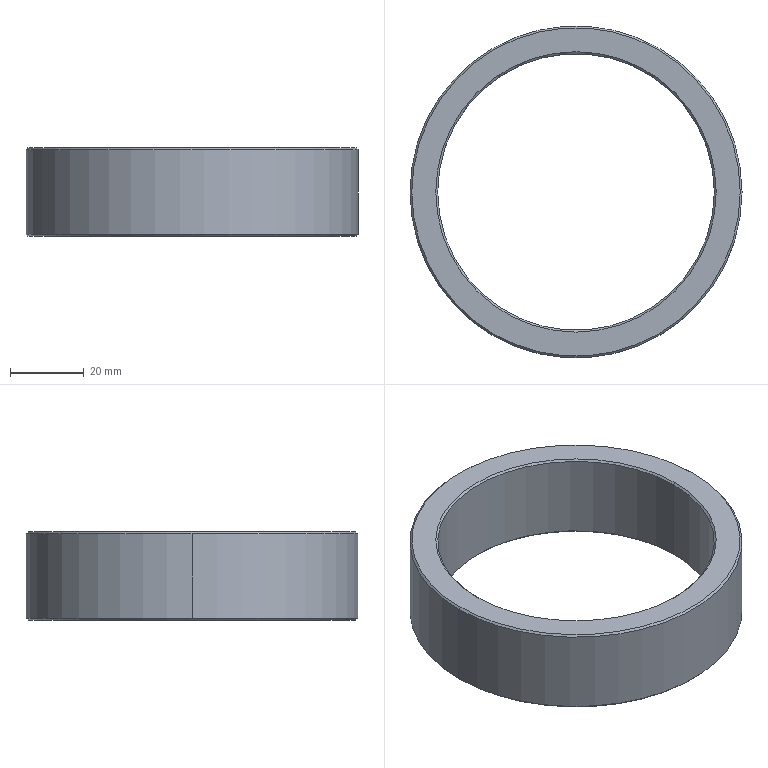Part | SolidWorks | features Chamfer 1, Extrusion 1 | 1 solid | 14 faces | box 90 x 90 x 24 mm | volume 46523 mm3 | cone 8 | cylinder 4 | plane 2 | commonest cylinder face diameters 75 x2 90 x2
STEP:
#1=CARTESIAN_POINT('',(44.5,0.,24.));
#2=VERTEX_POINT('',#1);
#3=CARTESIAN_POINT('',(-44.5,0.,24.));
#4=VERTEX_POINT('',#3);
#5=CARTESIAN_POINT('',(0.,0.,24.));
#6=DIRECTION('',(0.,0.,1.));
#7=DIRECTION('',(1.,0.,0.));
#8=AXIS2_PLACEMENT_3D('',#5,#6,#7);
#9=CIRCLE('',#8,44.5);
#10=EDGE_CURVE('',#2,#4,#9,.T.);
#11=ORIENTED_EDGE('',*,*,#10,.F.);
#12=CARTESIAN_POINT('',(45.,0.,23.5));
#13=VERTEX_POINT('',#12);
#14=CARTESIAN_POINT('',(44.5,0.,24.));
#15=DIRECTION('',(0.7071,0.,-0.7071));
#16=VECTOR('',#15,1000.);
#17=LINE('',#14,#16);
#18=EDGE_CURVE('',#2,#13,#17,.T.);
#19=ORIENTED_EDGE('',*,*,#18,.T.);
#20=CARTESIAN_POINT('',(-45.,0.,23.5));
#21=VERTEX_POINT('',#20);
#22=CARTESIAN_POINT('',(0.,0.,23.5));
#23=DIRECTION('',(0.,0.,-1.));
#24=DIRECTION('',(1.,0.,0.));
#25=AXIS2_PLACEMENT_3D('',#22,#23,#24);
#26=CIRCLE('',#25,45.);
#27=EDGE_CURVE('',#21,#13,#26,.T.);
#28=ORIENTED_EDGE('',*,*,#27,.F.);
#29=CARTESIAN_POINT('',(-44.5,0.,24.));
#30=DIRECTION('',(-0.7071,0.,-0.7071));
#31=VECTOR('',#30,1000.);
#32=LINE('',#29,#31);
#33=EDGE_CURVE('',#4,#21,#32,.T.);
#34=ORIENTED_EDGE('',*,*,#33,.F.);
#35=EDGE_LOOP('',(#11,#19,#28,#34));
#36=FACE_OUTER_BOUND('',#35,.T.);
#37=CARTESIAN_POINT('',(0.,0.,24.));
#38=DIRECTION('',(0.,0.,-1.));
#39=DIRECTION('',(-1.,0.,0.));
#40=AXIS2_PLACEMENT_3D('',#37,#38,#39);
#41=CONICAL_SURFACE('',#40,44.5,0.7854);
#42=ADVANCED_FACE('',(#36),#41,.T.);
#43=CARTESIAN_POINT('',(-37.5,0.,23.5));
#44=VERTEX_POINT('',#43);
#45=CARTESIAN_POINT('',(37.5,0.,23.5));
#46=VERTEX_POINT('',#45);
#47=CARTESIAN_POINT('',(0.,0.,23.5));
#48=DIRECTION('',(0.,0.,1.));
#49=DIRECTION('',(1.,0.,0.));
#50=AXIS2_PLACEMENT_3D('',#47,#48,#49);
#51=CIRCLE('',#50,37.5);
#52=EDGE_CURVE('',#44,#46,#51,.T.);
#53=ORIENTED_EDGE('',*,*,#52,.F.);
#54=CARTESIAN_POINT('',(-38.,0.,24.));
#55=VERTEX_POINT('',#54);
#56=CARTESIAN_POINT('',(-37.5,0.,23.5));
#57=DIRECTION('',(-0.7071,0.,0.7071));
#58=VECTOR('',#57,1000.);
#59=LINE('',#56,#58);
#60=EDGE_CURVE('',#44,#55,#59,.T.);
#61=ORIENTED_EDGE('',*,*,#60,.T.);
#62=CARTESIAN_POINT('',(38.,0.,24.));
#63=VERTEX_POINT('',#62);
#64=CARTESIAN_POINT('',(0.,0.,24.));
#65=DIRECTION('',(0.,0.,-1.));
#66=DIRECTION('',(1.,0.,0.));
#67=AXIS2_PLACEMENT_3D('',#64,#65,#66);
#68=CIRCLE('',#67,38.);
#69=EDGE_CURVE('',#63,#55,#68,.T.);
#70=ORIENTED_EDGE('',*,*,#69,.F.);
#71=CARTESIAN_POINT('',(37.5,0.,23.5));
#72=DIRECTION('',(0.7071,0.,0.7071));
#73=VECTOR('',#72,1000.);
#74=LINE('',#71,#73);
#75=EDGE_CURVE('',#46,#63,#74,.T.);
#76=ORIENTED_EDGE('',*,*,#75,.F.);
#77=EDGE_LOOP('',(#53,#61,#70,#76));
#78=FACE_OUTER_BOUND('',#77,.T.);
#79=CARTESIAN_POINT('',(0.,0.,23.5));
#80=DIRECTION('',(0.,0.,1.));
#81=DIRECTION('',(1.,0.,0.));
#82=AXIS2_PLACEMENT_3D('',#79,#80,#81);
#83=CONICAL_SURFACE('',#82,37.5,0.7854);
#84=ADVANCED_FACE('',(#78),#83,.F.);
#85=CARTESIAN_POINT('',(-44.5,0.,0.));
#86=VERTEX_POINT('',#85);
#87=CARTESIAN_POINT('',(44.5,0.,0.));
#88=VERTEX_POINT('',#87);
#89=CARTESIAN_POINT('',(0.,0.,0.));
#90=DIRECTION('',(0.,0.,-1.));
#91=DIRECTION('',(1.,0.,0.));
#92=AXIS2_PLACEMENT_3D('',#89,#90,#91);
#93=CIRCLE('',#92,44.5);
#94=EDGE_CURVE('',#86,#88,#93,.T.);
#95=ORIENTED_EDGE('',*,*,#94,.F.);
#96=CARTESIAN_POINT('',(-45.,0.,0.5));
#97=VERTEX_POINT('',#96);
#98=CARTESIAN_POINT('',(-45.,0.,0.5));
#99=DIRECTION('',(-0.7071,0.,0.7071));
#100=VECTOR('',#99,1000.);
#101=LINE('',#98,#100);
#102=EDGE_CURVE('',#86,#97,#101,.T.);
#103=ORIENTED_EDGE('',*,*,#102,.T.);
#104=CARTESIAN_POINT('',(45.,0.,0.5));
#105=VERTEX_POINT('',#104);
#106=CARTESIAN_POINT('',(0.,0.,0.5));
#107=DIRECTION('',(0.,0.,1.));
#108=DIRECTION('',(1.,0.,0.));
#109=AXIS2_PLACEMENT_3D('',#106,#107,#108);
#110=CIRCLE('',#109,45.);
#111=EDGE_CURVE('',#105,#97,#110,.T.);
#112=ORIENTED_EDGE('',*,*,#111,.F.);
#113=CARTESIAN_POINT('',(45.,0.,0.5));
#114=DIRECTION('',(0.7071,0.,0.7071));
#115=VECTOR('',#114,1000.);
#116=LINE('',#113,#115);
#117=EDGE_CURVE('',#88,#105,#116,.T.);
#118=ORIENTED_EDGE('',*,*,#117,.F.);
#119=EDGE_LOOP('',(#95,#103,#112,#118));
#120=FACE_OUTER_BOUND('',#119,.T.);
#121=CARTESIAN_POINT('',(0.,0.,0.5));
#122=DIRECTION('',(0.,0.,1.));
#123=DIRECTION('',(1.,0.,0.));
#124=AXIS2_PLACEMENT_3D('',#121,#122,#123);
#125=CONICAL_SURFACE('',#124,45.,0.7854);
#126=ADVANCED_FACE('',(#120),#125,.T.);
#127=CARTESIAN_POINT('',(37.5,0.,0.5));
#128=VERTEX_POINT('',#127);
#129=CARTESIAN_POINT('',(-37.5,0.,0.5));
#130=VERTEX_POINT('',#129);
#131=CARTESIAN_POINT('',(0.,0.,0.5));
#132=DIRECTION('',(0.,0.,-1.));
#133=DIRECTION('',(1.,0.,0.));
#134=AXIS2_PLACEMENT_3D('',#131,#132,#133);
#135=CIRCLE('',#134,37.5);
#136=EDGE_CURVE('',#128,#130,#135,.T.);
#137=ORIENTED_EDGE('',*,*,#136,.F.);
#138=CARTESIAN_POINT('',(38.,0.,0.));
#139=VERTEX_POINT('',#138);
#140=CARTESIAN_POINT('',(38.,0.,0.));
#141=DIRECTION('',(0.7071,0.,-0.7071));
#142=VECTOR('',#141,1000.);
#143=LINE('',#140,#142);
#144=EDGE_CURVE('',#128,#139,#143,.T.);
#145=ORIENTED_EDGE('',*,*,#144,.T.);
#146=CARTESIAN_POINT('',(-38.,0.,0.));
#147=VERTEX_POINT('',#146);
#148=CARTESIAN_POINT('',(0.,0.,0.));
#149=DIRECTION('',(0.,0.,1.));
#150=DIRECTION('',(1.,0.,0.));
#151=AXIS2_PLACEMENT_3D('',#148,#149,#150);
#152=CIRCLE('',#151,38.);
#153=EDGE_CURVE('',#147,#139,#152,.T.);
#154=ORIENTED_EDGE('',*,*,#153,.F.);
#155=CARTESIAN_POINT('',(-38.,0.,0.));
#156=DIRECTION('',(-0.7071,0.,-0.7071));
#157=VECTOR('',#156,1000.);
#158=LINE('',#155,#157);
#159=EDGE_CURVE('',#130,#147,#158,.T.);
#160=ORIENTED_EDGE('',*,*,#159,.F.);
#161=EDGE_LOOP('',(#137,#145,#154,#160));
#162=FACE_OUTER_BOUND('',#161,.T.);
#163=CARTESIAN_POINT('',(0.,0.,0.));
#164=DIRECTION('',(0.,0.,-1.));
#165=DIRECTION('',(-1.,0.,0.));
#166=AXIS2_PLACEMENT_3D('',#163,#164,#165);
#167=CONICAL_SURFACE('',#166,38.,0.7854);
#168=ADVANCED_FACE('',(#162),#167,.F.);
#169=ORIENTED_EDGE('',*,*,#52,.T.);
#170=CARTESIAN_POINT('',(37.5,0.,24.));
#171=DIRECTION('',(0.,0.,-1.));
#172=VECTOR('',#171,1000.);
#173=LINE('',#170,#172);
#174=EDGE_CURVE('',#46,#128,#173,.T.);
#175=ORIENTED_EDGE('',*,*,#174,.T.);
#176=ORIENTED_EDGE('',*,*,#136,.T.);
#177=CARTESIAN_POINT('',(-37.5,0.,24.));
#178=DIRECTION('',(0.,0.,-1.));
#179=VECTOR('',#178,1000.);
#180=LINE('',#177,#179);
#181=EDGE_CURVE('',#44,#130,#180,.T.);
#182=ORIENTED_EDGE('',*,*,#181,.F.);
#183=EDGE_LOOP('',(#169,#175,#176,#182));
#184=FACE_OUTER_BOUND('',#183,.T.);
#185=CARTESIAN_POINT('',(0.,0.,24.));
#186=DIRECTION('',(0.,0.,-1.));
#187=DIRECTION('',(-1.,0.,0.));
#188=AXIS2_PLACEMENT_3D('',#185,#186,#187);
#189=CYLINDRICAL_SURFACE('',#188,37.5);
#190=ADVANCED_FACE('',(#184),#189,.F.);
#191=ORIENTED_EDGE('',*,*,#27,.T.);
#192=CARTESIAN_POINT('',(45.,0.,24.));
#193=DIRECTION('',(0.,0.,-1.));
#194=VECTOR('',#193,1000.);
#195=LINE('',#192,#194);
#196=EDGE_CURVE('',#13,#105,#195,.T.);
#197=ORIENTED_EDGE('',*,*,#196,.T.);
#198=ORIENTED_EDGE('',*,*,#111,.T.);
#199=CARTESIAN_POINT('',(-45.,0.,24.));
#200=DIRECTION('',(0.,0.,-1.));
#201=VECTOR('',#200,1000.);
#202=LINE('',#199,#201);
#203=EDGE_CURVE('',#21,#97,#202,.T.);
#204=ORIENTED_EDGE('',*,*,#203,.F.);
#205=EDGE_LOOP('',(#191,#197,#198,#204));
#206=FACE_OUTER_BOUND('',#205,.T.);
#207=CARTESIAN_POINT('',(0.,0.,24.));
#208=DIRECTION('',(0.,0.,-1.));
#209=DIRECTION('',(-1.,0.,0.));
#210=AXIS2_PLACEMENT_3D('',#207,#208,#209);
#211=CYLINDRICAL_SURFACE('',#210,45.);
#212=ADVANCED_FACE('',(#206),#211,.T.);
#213=ORIENTED_EDGE('',*,*,#69,.T.);
#214=CARTESIAN_POINT('',(0.,0.,24.));
#215=DIRECTION('',(0.,0.,-1.));
#216=DIRECTION('',(1.,0.,0.));
#217=AXIS2_PLACEMENT_3D('',#214,#215,#216);
#218=CIRCLE('',#217,38.);
#219=EDGE_CURVE('',#55,#63,#218,.T.);
#220=ORIENTED_EDGE('',*,*,#219,.T.);
#221=EDGE_LOOP('',(#213,#220));
#222=FACE_BOUND('',#221,.T.);
#223=CARTESIAN_POINT('',(0.,0.,24.));
#224=DIRECTION('',(0.,0.,1.));
#225=DIRECTION('',(1.,0.,0.));
#226=AXIS2_PLACEMENT_3D('',#223,#224,#225);
#227=CIRCLE('',#226,44.5);
#228=EDGE_CURVE('',#4,#2,#227,.T.);
#229=ORIENTED_EDGE('',*,*,#228,.T.);
#230=ORIENTED_EDGE('',*,*,#10,.T.);
#231=EDGE_LOOP('',(#229,#230));
#232=FACE_OUTER_BOUND('',#231,.T.);
#233=CARTESIAN_POINT('',(0.,0.,24.));
#234=DIRECTION('',(0.,0.,1.));
#235=DIRECTION('',(1.,0.,0.));
#236=AXIS2_PLACEMENT_3D('',#233,#234,#235);
#237=PLANE('',#236);
#238=ADVANCED_FACE('',(#222,#232),#237,.T.);
#239=ORIENTED_EDGE('',*,*,#153,.T.);
#240=CARTESIAN_POINT('',(0.,0.,0.));
#241=DIRECTION('',(0.,0.,1.));
#242=DIRECTION('',(1.,0.,0.));
#243=AXIS2_PLACEMENT_3D('',#240,#241,#242);
#244=CIRCLE('',#243,38.);
#245=EDGE_CURVE('',#139,#147,#244,.T.);
#246=ORIENTED_EDGE('',*,*,#245,.T.);
#247=EDGE_LOOP('',(#239,#246));
#248=FACE_BOUND('',#247,.T.);
#249=CARTESIAN_POINT('',(0.,0.,0.));
#250=DIRECTION('',(0.,0.,-1.));
#251=DIRECTION('',(1.,0.,0.));
#252=AXIS2_PLACEMENT_3D('',#249,#250,#251);
#253=CIRCLE('',#252,44.5);
#254=EDGE_CURVE('',#88,#86,#253,.T.);
#255=ORIENTED_EDGE('',*,*,#254,.T.);
#256=ORIENTED_EDGE('',*,*,#94,.T.);
#257=EDGE_LOOP('',(#255,#256));
#258=FACE_OUTER_BOUND('',#257,.T.);
#259=CARTESIAN_POINT('',(0.,0.,0.));
#260=DIRECTION('',(0.,0.,1.));
#261=DIRECTION('',(1.,0.,0.));
#262=AXIS2_PLACEMENT_3D('',#259,#260,#261);
#263=PLANE('',#262);
#264=ADVANCED_FACE('',(#248,#258),#263,.F.);
#265=ORIENTED_EDGE('',*,*,#196,.F.);
#266=CARTESIAN_POINT('',(0.,0.,23.5));
#267=DIRECTION('',(0.,0.,-1.));
#268=DIRECTION('',(1.,0.,0.));
#269=AXIS2_PLACEMENT_3D('',#266,#267,#268);
#270=CIRCLE('',#269,45.);
#271=EDGE_CURVE('',#13,#21,#270,.T.);
#272=ORIENTED_EDGE('',*,*,#271,.T.);
#273=ORIENTED_EDGE('',*,*,#203,.T.);
#274=CARTESIAN_POINT('',(0.,0.,0.5));
#275=DIRECTION('',(0.,0.,1.));
#276=DIRECTION('',(1.,0.,0.));
#277=AXIS2_PLACEMENT_3D('',#274,#275,#276);
#278=CIRCLE('',#277,45.);
#279=EDGE_CURVE('',#97,#105,#278,.T.);
#280=ORIENTED_EDGE('',*,*,#279,.T.);
#281=EDGE_LOOP('',(#265,#272,#273,#280));
#282=FACE_OUTER_BOUND('',#281,.T.);
#283=CARTESIAN_POINT('',(0.,0.,24.));
#284=DIRECTION('',(0.,0.,-1.));
#285=DIRECTION('',(-1.,0.,0.));
#286=AXIS2_PLACEMENT_3D('',#283,#284,#285);
#287=CYLINDRICAL_SURFACE('',#286,45.);
#288=ADVANCED_FACE('',(#282),#287,.T.);
#289=ORIENTED_EDGE('',*,*,#174,.F.);
#290=CARTESIAN_POINT('',(0.,0.,23.5));
#291=DIRECTION('',(0.,0.,1.));
#292=DIRECTION('',(1.,0.,0.));
#293=AXIS2_PLACEMENT_3D('',#290,#291,#292);
#294=CIRCLE('',#293,37.5);
#295=EDGE_CURVE('',#46,#44,#294,.T.);
#296=ORIENTED_EDGE('',*,*,#295,.T.);
#297=ORIENTED_EDGE('',*,*,#181,.T.);
#298=CARTESIAN_POINT('',(0.,0.,0.5));
#299=DIRECTION('',(0.,0.,-1.));
#300=DIRECTION('',(1.,0.,0.));
#301=AXIS2_PLACEMENT_3D('',#298,#299,#300);
#302=CIRCLE('',#301,37.5);
#303=EDGE_CURVE('',#130,#128,#302,.T.);
#304=ORIENTED_EDGE('',*,*,#303,.T.);
#305=EDGE_LOOP('',(#289,#296,#297,#304));
#306=FACE_OUTER_BOUND('',#305,.T.);
#307=CARTESIAN_POINT('',(0.,0.,24.));
#308=DIRECTION('',(0.,0.,-1.));
#309=DIRECTION('',(-1.,0.,0.));
#310=AXIS2_PLACEMENT_3D('',#307,#308,#309);
#311=CYLINDRICAL_SURFACE('',#310,37.5);
#312=ADVANCED_FACE('',(#306),#311,.F.);
#313=ORIENTED_EDGE('',*,*,#144,.F.);
#314=ORIENTED_EDGE('',*,*,#303,.F.);
#315=ORIENTED_EDGE('',*,*,#159,.T.);
#316=ORIENTED_EDGE('',*,*,#245,.F.);
#317=EDGE_LOOP('',(#313,#314,#315,#316));
#318=FACE_OUTER_BOUND('',#317,.T.);
#319=CARTESIAN_POINT('',(0.,0.,0.));
#320=DIRECTION('',(0.,0.,-1.));
#321=DIRECTION('',(-1.,0.,0.));
#322=AXIS2_PLACEMENT_3D('',#319,#320,#321);
#323=CONICAL_SURFACE('',#322,38.,0.7854);
#324=ADVANCED_FACE('',(#318),#323,.F.);
#325=ORIENTED_EDGE('',*,*,#102,.F.);
#326=ORIENTED_EDGE('',*,*,#254,.F.);
#327=ORIENTED_EDGE('',*,*,#117,.T.);
#328=ORIENTED_EDGE('',*,*,#279,.F.);
#329=EDGE_LOOP('',(#325,#326,#327,#328));
#330=FACE_OUTER_BOUND('',#329,.T.);
#331=CARTESIAN_POINT('',(0.,0.,0.5));
#332=DIRECTION('',(0.,0.,1.));
#333=DIRECTION('',(1.,0.,0.));
#334=AXIS2_PLACEMENT_3D('',#331,#332,#333);
#335=CONICAL_SURFACE('',#334,45.,0.7854);
#336=ADVANCED_FACE('',(#330),#335,.T.);
#337=ORIENTED_EDGE('',*,*,#60,.F.);
#338=ORIENTED_EDGE('',*,*,#295,.F.);
#339=ORIENTED_EDGE('',*,*,#75,.T.);
#340=ORIENTED_EDGE('',*,*,#219,.F.);
#341=EDGE_LOOP('',(#337,#338,#339,#340));
#342=FACE_OUTER_BOUND('',#341,.T.);
#343=CARTESIAN_POINT('',(0.,0.,23.5));
#344=DIRECTION('',(0.,0.,1.));
#345=DIRECTION('',(1.,0.,0.));
#346=AXIS2_PLACEMENT_3D('',#343,#344,#345);
#347=CONICAL_SURFACE('',#346,37.5,0.7854);
#348=ADVANCED_FACE('',(#342),#347,.F.);
#349=ORIENTED_EDGE('',*,*,#18,.F.);
#350=ORIENTED_EDGE('',*,*,#228,.F.);
#351=ORIENTED_EDGE('',*,*,#33,.T.);
#352=ORIENTED_EDGE('',*,*,#271,.F.);
#353=EDGE_LOOP('',(#349,#350,#351,#352));
#354=FACE_OUTER_BOUND('',#353,.T.);
#355=CARTESIAN_POINT('',(0.,0.,24.));
#356=DIRECTION('',(0.,0.,-1.));
#357=DIRECTION('',(-1.,0.,0.));
#358=AXIS2_PLACEMENT_3D('',#355,#356,#357);
#359=CONICAL_SURFACE('',#358,44.5,0.7854);
#360=ADVANCED_FACE('',(#354),#359,.T.);
#361=CLOSED_SHELL('',(#42,#84,#126,#168,#190,#212,#238,#264,#288,#312,#324,#336,#348,#360));
#362=MANIFOLD_SOLID_BREP('',#361);
#363=CARTESIAN_POINT('',(0.,0.,0.));
#364=DIRECTION('',(0.,0.,1.));
#365=DIRECTION('',(1.,0.,0.));
#366=AXIS2_PLACEMENT_3D('',#363,#364,#365);
#367=(LENGTH_UNIT()NAMED_UNIT(*)SI_UNIT(.MILLI.,.METRE.));
#368=UNCERTAINTY_MEASURE_WITH_UNIT(LENGTH_MEASURE(0.00001),#367,'','');
#369=(NAMED_UNIT(*)PLANE_ANGLE_UNIT()SI_UNIT($,.RADIAN.));
#370=(NAMED_UNIT(*)SI_UNIT($,.STERADIAN.)SOLID_ANGLE_UNIT());
#371=(GEOMETRIC_REPRESENTATION_CONTEXT(3)GLOBAL_UNCERTAINTY_ASSIGNED_CONTEXT((#368))GLOBAL_UNIT_ASSIGNED_CONTEXT((#367,#369,#370))REPRESENTATION_CONTEXT('',''));
#372=ADVANCED_BREP_SHAPE_REPRESENTATION('',(#362,#366),#371);